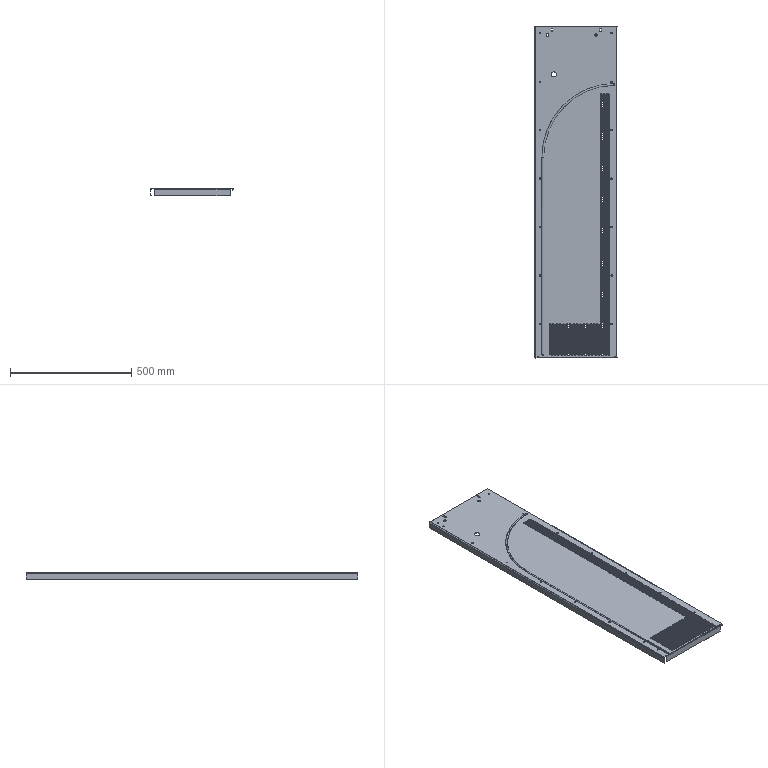Part | STEP file | 64635212 | 1 solid | 2780 faces | box 342.5 x 1370 x 32 mm | volume 739959 mm3 | cylinder 2601 | plane 165 | torus 10 | sphere 4 | commonest cylinder face diameters 6 x2578 4 x5 5 x4 10 x4 1 x2 3 x2